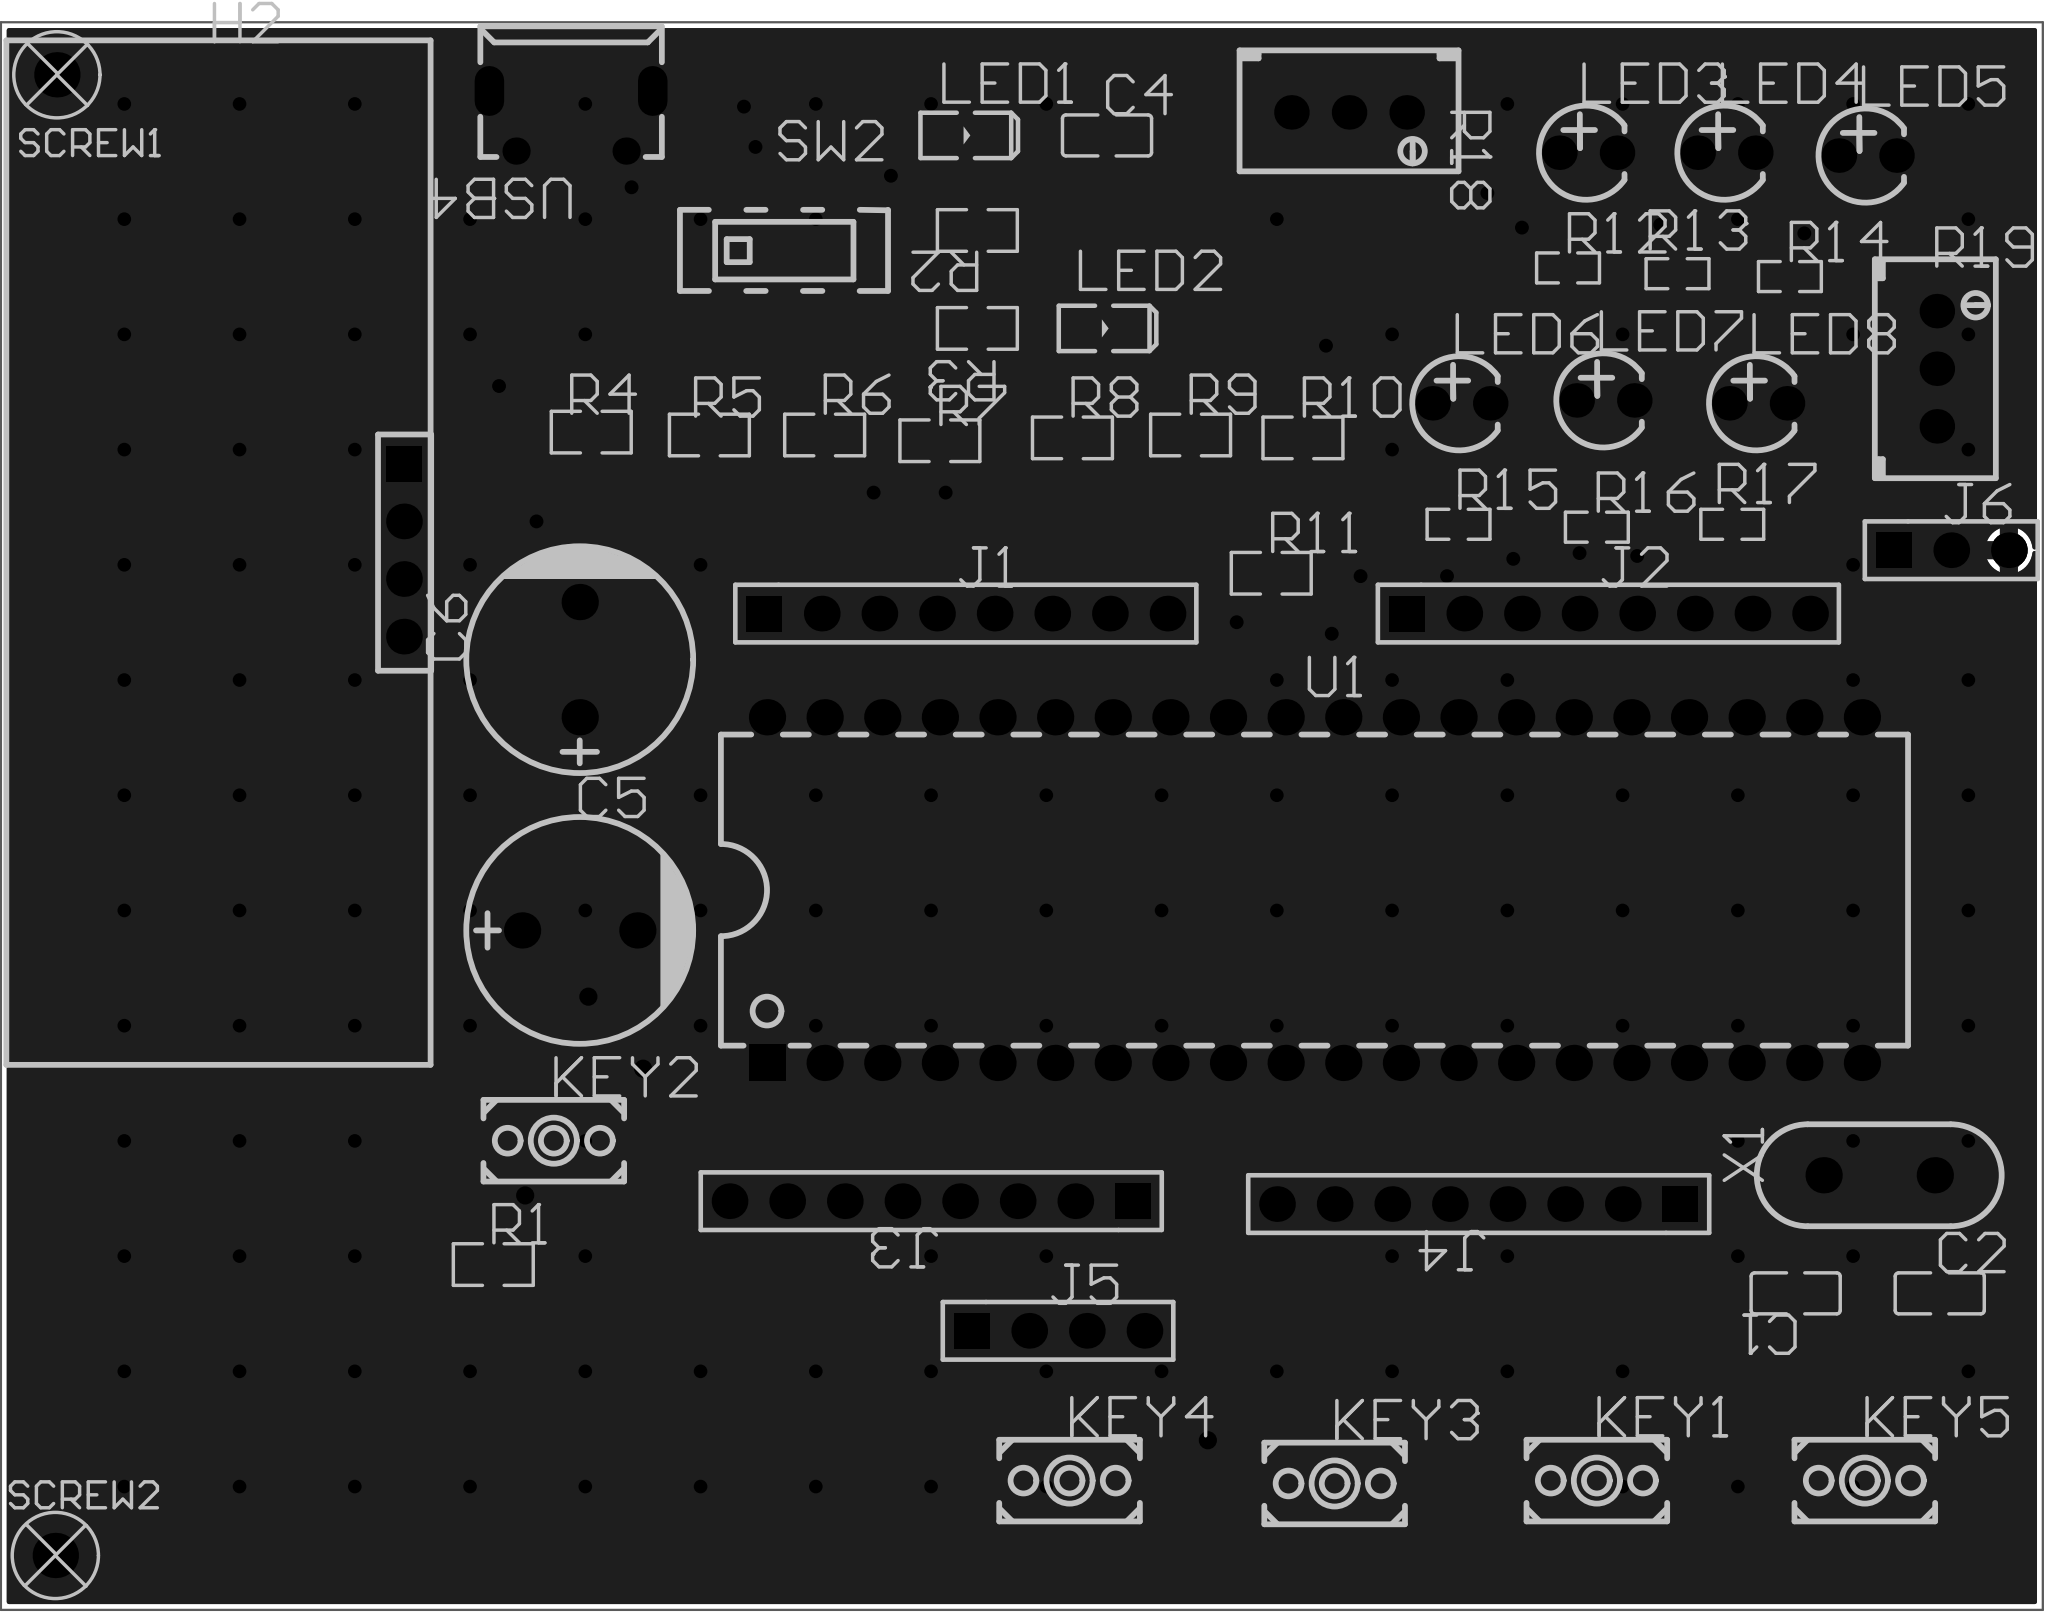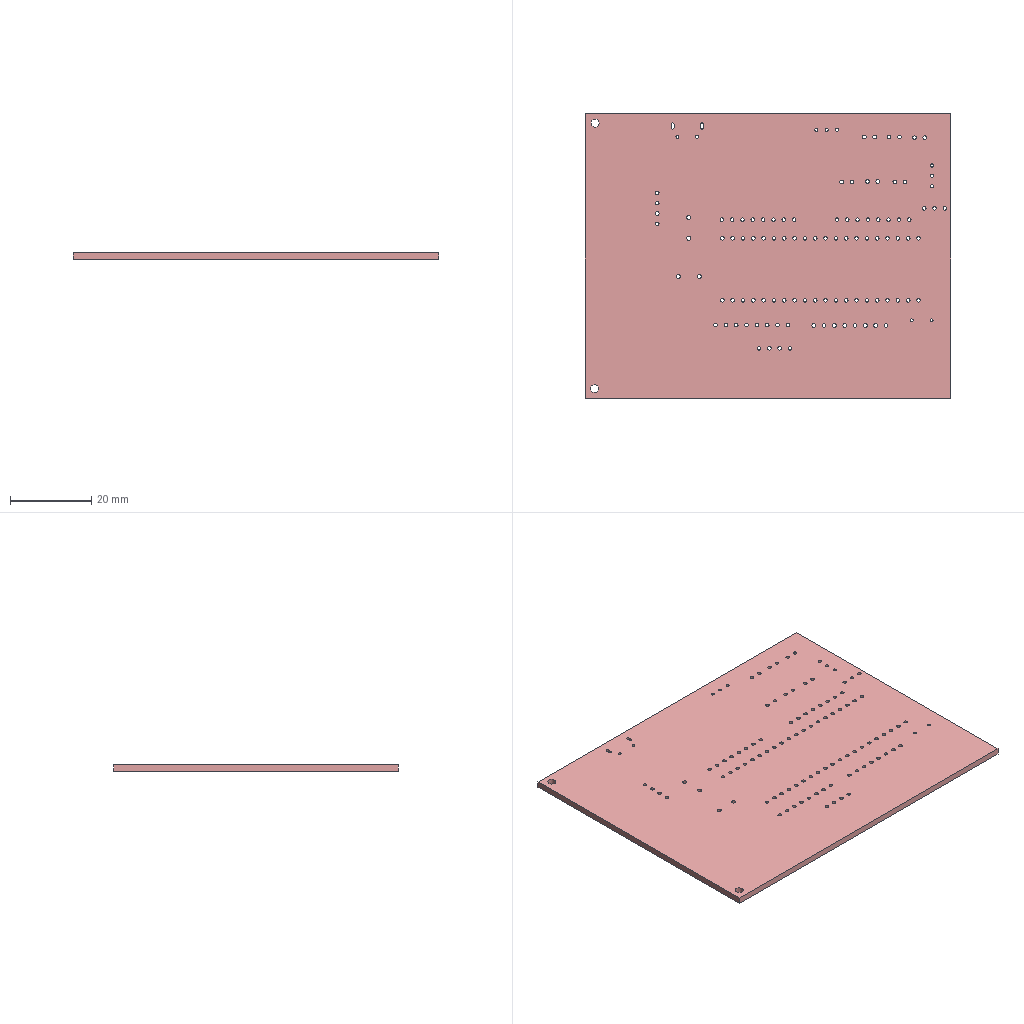Circuit board layout | Altium Designer | box 90 x 70 x 1.6 mm
Layer stack:
# Altium Designer layer stack of  (unit mm; dielectric type: 0 none, 1 core, 2 prepreg, 3 surface material)
index,name,kind,layer,copper_thickness_mm,dielectric_type,dielectric_thickness_mm,dielectric_material,dielectric_constant
0,Top Paste Mask Layer,other,,,,,,
1,Top Silkscreen Layer,other,,,,,,
2,Top Solder Mask Layer,dielectric,,,3,0.01,,3.3
3,Top Layer,copper,Top Layer,0.035,,,,
4,Dielectric1,dielectric,,,3,1.51,FR4,4.5
5,Bottom Layer,copper,Bottom Layer,0.035,,,,
6,Bottom Solder Mask Layer,dielectric,,,3,0.01,,3.3
7,Bottom Silkscreen Layer,other,,,,,,
8,Bottom Paste Mask Layer,other,,,,,,
# drill layer pairs: low layer,high layer
drill_pair,Top Layer,Bottom Layer
Part placement:
Designator,Comment,Layer,Footprint,Center-X(mm),Center-Y(mm),Rotation
C1,33p,TopLayer,C0805,163.957,95.377,180
C2,33p,TopLayer,C0805,170.307,95.377,0
C4,10NF,TopLayer,C0805,133.604,146.431,0
C5,10uF,TopLayer,CAP-TH_BD10.0-P5.00-D1.0-FD,110.363,111.379,0
C6,10uF,TopLayer,CAP-TH_BD10.0-P5.00-D1.0-FD,110.363,123.317,90
H2,HC-SR04,TopLayer,HC-SR04,102.616,128.143,0
J1,HDR-M-2.54_1x8,TopLayer,HDR-M-2.54_1X8,127.381,125.349,0
J2,HDR-M-2.54_1x8,TopLayer,HDR-M-2.54_1X8,155.702,125.349,0
J3,HDR-M-2.54_1x8,TopLayer,HDR-M-2.54_1X8,125.857,99.441,180
J4,HDR-M-2.54_1x8,TopLayer,HDR-M-2.54_1X8,149.987,99.314,180
J5,HDR-M-2.54_1x4,TopLayer,HDR-M-2.54_1X4,131.445,93.726,0
J6,HDR-M-2.54_1x3,TopLayer,HDR-M-2.54_1X3,170.815,128.143,0
KEY1,K2-3.6×6.1_SMD,TopLayer,KEY-SMD_2P-L6.2-W3.6-LS8.0,155.194,87.122,0
KEY2,K2-3.6×6.1_SMD,TopLayer,KEY-SMD_2P-L6.2-W3.6-LS8.0,109.22,102.108,0
KEY3,K2-3.6×6.1_SMD,TopLayer,KEY-SMD_2P-L6.2-W3.6-LS8.0,143.637,86.995,0
KEY4,K2-3.6×6.1_SMD,TopLayer,KEY-SMD_2P-L6.2-W3.6-LS8.0,131.953,87.122,0
KEY5,K2-3.6×6.1_SMD,TopLayer,KEY-SMD_2P-L6.2-W3.6-LS8.0,167.005,87.122,0
LED1,LED-0805_R,TopLayer,LED0805_RED,127.381,146.431,0
LED2,LED-0805_R,TopLayer,LED0805_RED,133.477,137.922,0
LED3,204-10SDRD/S530-A3-L,TopLayer,LED-TH_BD3.8-P2.54-FD,154.813,145.669,0
LED4,204-10SDRD/S530-A3-L,TopLayer,LED-TH_BD3.8-P2.54-FD,160.909,145.669,0
LED5,204-10SDRD/S530-A3-L,TopLayer,LED-TH_BD3.8-P2.54-FD,167.132,145.542,0
LED6,204-10SDRD/S530-A3-L,TopLayer,LED-TH_BD3.8-P2.54-FD,149.225,134.62,0
LED7,204-10SDRD/S530-A3-L,TopLayer,LED-TH_BD3.8-P2.54-FD,155.575,134.747,0
LED8,204-10SDRD/S530-A3-L,TopLayer,LED-TH_BD3.8-P2.54-FD,162.306,134.62,0
R1,10k,TopLayer,R0805,106.553,96.647,0
R2,1.5k,TopLayer,R0805,127.889,142.24,180
R3,1k,TopLayer,R0805,127.889,137.922,180
R4,4.7k,TopLayer,R0805,110.871,133.35,180
R5,4.7k,TopLayer,R0805,116.078,133.223,180
R6,4.7k,TopLayer,R0805,121.158,133.223,0
R7,4.7k,TopLayer,R0805,126.238,132.969,0
R8,4.7k,TopLayer,R0805,132.08,133.096,0
R9,4.7k,TopLayer,R0805,137.287,133.223,0
R10,4.7k,TopLayer,R0805,142.24,133.096,0
R11,4.7k,TopLayer,R0805,140.843,127.127,0
R12,1000,TopLayer,R0603,153.924,140.589,0
R13,1000,TopLayer,R0603,158.75,140.335,0
R14,1000,TopLayer,R0603,163.703,140.208,0
R15,1000,TopLayer,R0603,149.098,129.286,0
R16,1000,TopLayer,R0603,155.194,129.159,0
R17,1000,TopLayer,R0603,161.163,129.286,0
R18,10kΩ,TopLayer,RES-ADJ-TH_3296W,144.272,147.447,270
R19,10kΩ,TopLayer,RES-ADJ-TH_3296W,170.18,136.144,0
SW2,MST22D18G2 125,TopLayer,SW-SMD_MST22D18G2,119.38,141.351,0
U1,STC90C52RC-40I_C14023,TopLayer,DIP-40_L52.0-W13.7-P2.54-LS15.2-BL,142.748,113.157,0
USB4,USB-Micro_1,TopLayer,MICRO-USB-SMD_5P-P0.65-H-F_C10418,109.982,147.066,180
X1,11.059MHz,TopLayer,OSC-TH_L10.0-W4.5-P5.00,167.64,100.584,90
SCREW1,,TopLayer,M2螺丝,87.318,149.104,0
SCREW2,,TopLayer,M2螺丝,87.249,83.82,0
Pad and via stacks:
# Altium Designer via and pad stacks of  (unit mm). Each distinct definition once, with the count of objects using it.
# via: kind,start_layer,end_layer,hole_mm,diameter_mm,mode(0 simple;1 top-mid-bottom;2 full stack),diameter_per_layer,count,example_net
# pad: kind,layer,hole_mm,hole_type(0 round;1 square;2 slot),plating,top_size,top_shape(1 round;2 rect;3 octagon;9 rounded rect),mid_size,bottom_size,mode,footprint,size_per_layer,count,example
pad,Top Layer,0,0,plated,1.41x1.35,2,1.41x1.35,1.41x1.35,0,C0805,,6,C1.2
pad,Top Layer,0,0,plated,1.5x1.4,2,1.5x1.4,1.5x1.4,0,KEY-SMD_2P-L6.2-W3.6-LS8.0,,10,KEY1.1
pad,Top Layer,0,0,plated,1.3x1.399,2,1.3x1.399,1.3x1.399,0,LED0805_RED,,4,LED1.1
pad,Top Layer,0,0,plated,1.133x1.377,2,1.133x1.377,1.133x1.377,0,R0805,,22,R1.2
pad,Top Layer,0,0,plated,0.8065x0.864,2,0.8065x0.864,0.8065x0.864,0,R0603,,12,R12.2
pad,Top Layer,0,0,plated,1.2x2,2,1.2x2,1.2x2,0,SW-SMD_MST22D18G2,,6,SW2.5
pad,Top Layer,0,0,plated,1.25x0.4,2,1.25x0.4,1.25x0.4,0,MICRO-USB-SMD_5P-P0.65-H-F_C10418,,5,USB4.5
pad,Multi-Layer,1,0,plated,1.6x1.6,1,1.6x1.6,1.6x1.6,0,CAP-TH_BD10.0-P5.00-D1.0-FD,,4,C5.1
pad,Multi-Layer,0.889,0,plated,1.575x1.575,1,1.575x1.575,1.575x1.575,0,HC-SR04,,3,H2.4
pad,Multi-Layer,0.889,0,plated,1.575x1.575,2,1.575x1.575,1.575x1.575,0,HC-SR04,,1,H2.1
pad,Multi-Layer,0.889,0,plated,1.575x1.575,2,1.575x1.575,1.575x1.575,0,HDR-M-2.54_1X8,,4,J1.1
pad,Multi-Layer,0.889,0,plated,1.575x1.575,1,1.575x1.575,1.575x1.575,0,HDR-M-2.54_1X8,,28,J1.2
pad,Multi-Layer,0.889,0,plated,1.575x1.575,2,1.575x1.575,1.575x1.575,0,HDR-M-2.54_1X4,,1,J5.1
pad,Multi-Layer,0.889,0,plated,1.575x1.575,1,1.575x1.575,1.575x1.575,0,HDR-M-2.54_1X4,,3,J5.2
pad,Multi-Layer,0.889,0,plated,1.575x1.575,1,1.575x1.575,1.575x1.575,0,HDR-M-2.54_1X3,,2,J6.3
pad,Multi-Layer,0.889,0,plated,1.575x1.575,2,1.575x1.575,1.575x1.575,0,HDR-M-2.54_1X3,,1,J6.1
pad,Multi-Layer,0.9,0,plated,1.524x1.524,1,1.524x1.524,1.524x1.524,0,LED-TH_BD3.8-P2.54-FD,,12,LED3.2
pad,Multi-Layer,0.762,0,plated,1.524x1.524,1,1.524x1.524,1.524x1.524,0,RES-ADJ-TH_3296W,,6,R18.2
pad,Multi-Layer,0.889,0,plated,1.6x1.6,1,1.6x1.6,1.6x1.6,0,DIP-40_L52.0-W13.7-P2.54-LS15.2-BL,,39,U1.31
pad,Multi-Layer,0.889,0,plated,1.6x1.6,2,1.6x1.6,1.6x1.6,0,DIP-40_L52.0-W13.7-P2.54-LS15.2-BL,,1,U1.1
pad,Multi-Layer,0.7,2,plated,1.3x2.2,1,1.3x2.2,1.3x2.2,0,MICRO-USB-SMD_5P-P0.65-H-F_C10418,,2,USB4.SH2
pad,Multi-Layer,0.7,0,plated,1.2x1.2,1,1.2x1.2,1.2x1.2,0,MICRO-USB-SMD_5P-P0.65-H-F_C10418,,2,USB4.SH0
pad,Multi-Layer,0.7,0,plated,1.6x1.6,1,1.6x1.6,1.6x1.6,0,OSC-TH_L10.0-W4.5-P5.00,,2,X1.2
pad,Multi-Layer,2,0,plated,2x2,1,2x2,2x2,0,M2\u00C2\u00DD\u00CB\u00BF,,2,SCREW1.1
via,Top Layer,Bottom Layer,0.3048,0.6096,0,,20,$1N557
via,Top Layer,Bottom Layer,0.5004,0.8,0,,4,RST
via,Top Layer,Bottom Layer,0.3048,0.6,0,,145,GND
Copper pours:
name,layer,net,type(0 solid;1 hatched;2 none)
Bottom Layer-GND,Bottom Layer,GND,0
Top Layer-GND,Top Layer,GND,0
Design rules, without the lines most boards share:
# Altium Designer design rules of  (exported by Altium Designer, unit mm)
# columns: name | kind | enabled | priority | scope1 | scope2 | descriptor | typed fields (field=value)
Power | 0 | disabled | 1 | All | All | Clearance Constraint (Gap=11.811mil) (Disabled)(All),(All) | gap=0.3
Power_1 | 63 | disabled | 1 | All | All | Board Clearance Constraint (Gap=0mil) (Disabled)(All) |
Plane_Default | 0 | disabled | 2 | All | All | Clearance Constraint (Gap=5.984mil) (Disabled)(All),(All) | gap=0.152
Plane_Default_1 | 63 | disabled | 2 | All | All | Board Clearance Constraint (Gap=0mil) (Disabled)(All) |
Plane_Power | 0 | disabled | 3 | All | All | Clearance Constraint (Gap=5.984mil) (Disabled)(All),(All) | gap=0.152
Plane_Power_1 | 63 | disabled | 3 | All | All | Board Clearance Constraint (Gap=0mil) (Disabled)(All) |
Copper_gge8343 | 0 | disabled | 4 | All | All | Clearance Constraint (Gap=5.984mil) (Disabled)(All),(All) | gap=0.152
Copper_gge8343_1 | 63 | disabled | 4 | All | All | Board Clearance Constraint (Gap=0mil) (Disabled)(All) |
Copper_gge8337 | 0 | disabled | 5 | All | All | Clearance Constraint (Gap=5.984mil) (Disabled)(All),(All) | gap=0.152
Copper_gge8337_1 | 63 | disabled | 5 | All | All | Board Clearance Constraint (Gap=0mil) (Disabled)(All) |
Default | 0 | enabled | 6 | All | All | Clearance Constraint (Gap=5.984mil) (All),(All) | gap=0.152
Default_1 | 63 | enabled | 6 | All | All | Board Clearance Constraint (Gap=0mil) (All) |
otherClearance | 52 | enabled | 1 | All | All | Hole To Hole Clearance (Gap=11.8mil) (All),(All) | gap=0.2997
Power_2 | 2 | disabled | 1 | All | All | Width Constraint (Min=19.7mil) (Max=1000mil) (Preferred=19.7mil) (Disabled)(All) |
Default_2 | 2 | enabled | 2 | All | All | Width Constraint (Min=10mil) (Max=1000mil) (Preferred=10mil) (All) |
Power_3 | 11 | disabled | 1 | All | All | Routing Via (MinHoleWidth=11.811mil) (MaxHoleWidth=2362mil) (PreferredHoleWidth=11.811mil) (MinWidth=23.622mil) (MaxWidth=3938mil) (PreferedWidth=23.622mil) (Disabled)(All) | via_min_hole=0.3 via_max_hole=59.995 via_preferred_diameter=0.6 via_preferred_hole=0.3
Default_3 | 11 | enabled | 2 | All | All | Routing Via (MinHoleWidth=12.008mil) (MaxHoleWidth=2362mil) (PreferredHoleWidth=12.008mil) (MinWidth=23.622mil) (MaxWidth=3938mil) (PreferedWidth=23.622mil) (All) | via_min_hole=0.305 via_max_hole=59.995 via_preferred_diameter=0.6 via_preferred_hole=0.305
Power_4 | 6 | disabled | 1 | All | All | Power Plane Connect Rule(Relief Connect )(Expansion=20mil) (Conductor Width=0mil) (Air Gap=10mil) (Entries=4) (Disabled)(All) | relief_conductor_width=0 relief_entries=4 relief_expansion=0.508
Default_4 | 6 | enabled | 2 | All | All | Power Plane Connect Rule(Relief Connect )(Expansion=20mil) (Conductor Width=0mil) (Air Gap=10mil) (Entries=4) (All) | relief_conductor_width=0 relief_entries=4 relief_expansion=0.508
gge8337 | 20 | disabled | 1 | All | All | Polygon Connect Rule(Relief Connect )(Conductor Width=0mil) (Relief Angle=90 Angle) (Entries=4) (Air Gap Width=10mil) (Disabled)(All),(All) | connect_style(0=relief,1=direct,2=none)=0 relief_conductor_width=0 relief_entries=4
gge8343 | 20 | enabled | 2 | All | All | Polygon Connect Rule(Relief Connect )(Conductor Width=0mil) (Relief Angle=90 Angle) (Entries=4) (Air Gap Width=10mil) (All),(All) | connect_style(0=relief,1=direct,2=none)=0 relief_conductor_width=0 relief_entries=4